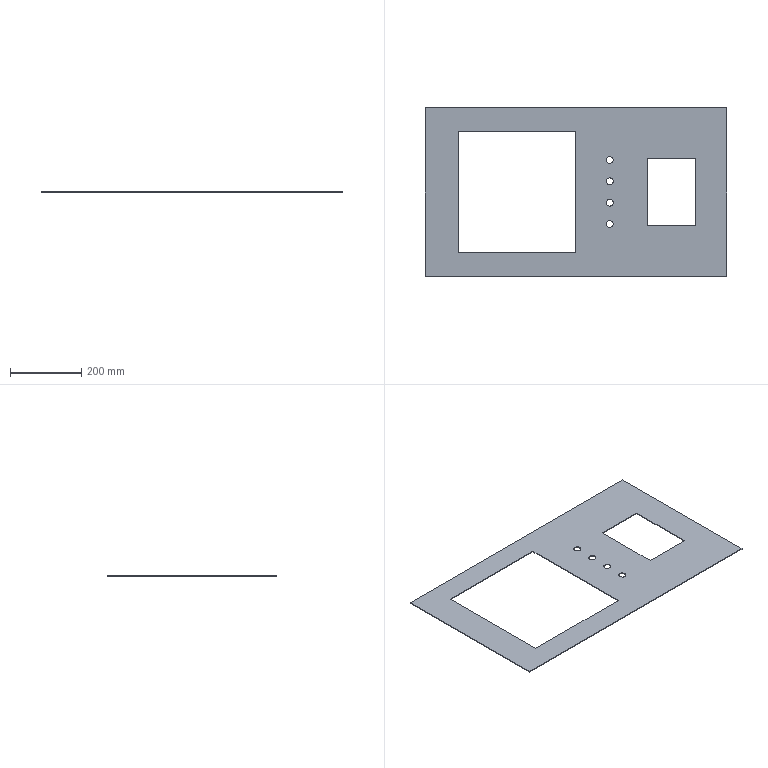Part | STEP file | Upper frame door panel | 1 solid | 22 faces | box 848 x 474.5 x 2 mm | volume 525505 mm3 | plane 14 | cylinder 8 | commonest cylinder face diameters 20 x8
STEP:
#1=CARTESIAN_POINT('',(105.,90.,0.));
#2=VERTEX_POINT('',#1);
#3=CARTESIAN_POINT('',(85.,90.,0.));
#4=VERTEX_POINT('',#3);
#5=CARTESIAN_POINT('',(95.,90.,0.));
#6=DIRECTION('',(0.,0.,-1.));
#7=DIRECTION('',(-1.,0.,0.));
#8=AXIS2_PLACEMENT_3D('',#5,#6,#7);
#9=CIRCLE('',#8,10.);
#10=EDGE_CURVE('',#2,#4,#9,.T.);
#11=ORIENTED_EDGE('',*,*,#10,.T.);
#12=CARTESIAN_POINT('',(85.,90.,2.));
#13=VERTEX_POINT('',#12);
#14=CARTESIAN_POINT('',(85.,90.,-0.001));
#15=DIRECTION('',(0.,0.,1.));
#16=VECTOR('',#15,1000.);
#17=LINE('',#14,#16);
#18=EDGE_CURVE('',#4,#13,#17,.T.);
#19=ORIENTED_EDGE('',*,*,#18,.T.);
#20=CARTESIAN_POINT('',(105.,90.,2.));
#21=VERTEX_POINT('',#20);
#22=CARTESIAN_POINT('',(95.,90.,2.));
#23=DIRECTION('',(0.,0.,-1.));
#24=DIRECTION('',(1.,0.,0.));
#25=AXIS2_PLACEMENT_3D('',#22,#23,#24);
#26=CIRCLE('',#25,10.);
#27=EDGE_CURVE('',#21,#13,#26,.T.);
#28=ORIENTED_EDGE('',*,*,#27,.F.);
#29=CARTESIAN_POINT('',(105.,90.,-0.001));
#30=DIRECTION('',(0.,0.,1.));
#31=VECTOR('',#30,1000.);
#32=LINE('',#29,#31);
#33=EDGE_CURVE('',#2,#21,#32,.T.);
#34=ORIENTED_EDGE('',*,*,#33,.F.);
#35=EDGE_LOOP('',(#11,#19,#28,#34));
#36=FACE_OUTER_BOUND('',#35,.T.);
#37=CARTESIAN_POINT('',(95.,90.,-0.001));
#38=DIRECTION('',(0.,0.,1.));
#39=DIRECTION('',(1.,0.,0.));
#40=AXIS2_PLACEMENT_3D('',#37,#38,#39);
#41=CYLINDRICAL_SURFACE('',#40,10.);
#42=ADVANCED_FACE('',(#36),#41,.F.);
#43=CARTESIAN_POINT('',(105.,30.,0.));
#44=VERTEX_POINT('',#43);
#45=CARTESIAN_POINT('',(85.,30.,0.));
#46=VERTEX_POINT('',#45);
#47=CARTESIAN_POINT('',(95.,30.,0.));
#48=DIRECTION('',(0.,0.,-1.));
#49=DIRECTION('',(-1.,0.,0.));
#50=AXIS2_PLACEMENT_3D('',#47,#48,#49);
#51=CIRCLE('',#50,10.);
#52=EDGE_CURVE('',#44,#46,#51,.T.);
#53=ORIENTED_EDGE('',*,*,#52,.T.);
#54=CARTESIAN_POINT('',(85.,30.,2.));
#55=VERTEX_POINT('',#54);
#56=CARTESIAN_POINT('',(85.,30.,-0.001));
#57=DIRECTION('',(0.,0.,1.));
#58=VECTOR('',#57,1000.);
#59=LINE('',#56,#58);
#60=EDGE_CURVE('',#46,#55,#59,.T.);
#61=ORIENTED_EDGE('',*,*,#60,.T.);
#62=CARTESIAN_POINT('',(105.,30.,2.));
#63=VERTEX_POINT('',#62);
#64=CARTESIAN_POINT('',(95.,30.,2.));
#65=DIRECTION('',(0.,0.,-1.));
#66=DIRECTION('',(1.,0.,0.));
#67=AXIS2_PLACEMENT_3D('',#64,#65,#66);
#68=CIRCLE('',#67,10.);
#69=EDGE_CURVE('',#63,#55,#68,.T.);
#70=ORIENTED_EDGE('',*,*,#69,.F.);
#71=CARTESIAN_POINT('',(105.,30.,-0.001));
#72=DIRECTION('',(0.,0.,1.));
#73=VECTOR('',#72,1000.);
#74=LINE('',#71,#73);
#75=EDGE_CURVE('',#44,#63,#74,.T.);
#76=ORIENTED_EDGE('',*,*,#75,.F.);
#77=EDGE_LOOP('',(#53,#61,#70,#76));
#78=FACE_OUTER_BOUND('',#77,.T.);
#79=CARTESIAN_POINT('',(95.,30.,-0.001));
#80=DIRECTION('',(0.,0.,1.));
#81=DIRECTION('',(1.,0.,0.));
#82=AXIS2_PLACEMENT_3D('',#79,#80,#81);
#83=CYLINDRICAL_SURFACE('',#82,10.);
#84=ADVANCED_FACE('',(#78),#83,.F.);
#85=CARTESIAN_POINT('',(85.,-30.,0.));
#86=VERTEX_POINT('',#85);
#87=CARTESIAN_POINT('',(105.,-30.,0.));
#88=VERTEX_POINT('',#87);
#89=CARTESIAN_POINT('',(95.,-30.,0.));
#90=DIRECTION('',(0.,0.,1.));
#91=DIRECTION('',(-1.,0.,0.));
#92=AXIS2_PLACEMENT_3D('',#89,#90,#91);
#93=CIRCLE('',#92,10.);
#94=EDGE_CURVE('',#86,#88,#93,.T.);
#95=ORIENTED_EDGE('',*,*,#94,.F.);
#96=CARTESIAN_POINT('',(85.,-30.,2.));
#97=VERTEX_POINT('',#96);
#98=CARTESIAN_POINT('',(85.,-30.,-0.001));
#99=DIRECTION('',(0.,0.,1.));
#100=VECTOR('',#99,1000.);
#101=LINE('',#98,#100);
#102=EDGE_CURVE('',#86,#97,#101,.T.);
#103=ORIENTED_EDGE('',*,*,#102,.T.);
#104=CARTESIAN_POINT('',(105.,-30.,2.));
#105=VERTEX_POINT('',#104);
#106=CARTESIAN_POINT('',(95.,-30.,2.));
#107=DIRECTION('',(0.,0.,1.));
#108=DIRECTION('',(1.,0.,0.));
#109=AXIS2_PLACEMENT_3D('',#106,#107,#108);
#110=CIRCLE('',#109,10.);
#111=EDGE_CURVE('',#97,#105,#110,.T.);
#112=ORIENTED_EDGE('',*,*,#111,.T.);
#113=CARTESIAN_POINT('',(105.,-30.,-0.001));
#114=DIRECTION('',(0.,0.,1.));
#115=VECTOR('',#114,1000.);
#116=LINE('',#113,#115);
#117=EDGE_CURVE('',#88,#105,#116,.T.);
#118=ORIENTED_EDGE('',*,*,#117,.F.);
#119=EDGE_LOOP('',(#95,#103,#112,#118));
#120=FACE_OUTER_BOUND('',#119,.T.);
#121=CARTESIAN_POINT('',(95.,-30.,-0.001));
#122=DIRECTION('',(0.,0.,1.));
#123=DIRECTION('',(1.,0.,0.));
#124=AXIS2_PLACEMENT_3D('',#121,#122,#123);
#125=CYLINDRICAL_SURFACE('',#124,10.);
#126=ADVANCED_FACE('',(#120),#125,.F.);
#127=CARTESIAN_POINT('',(85.,-90.,0.));
#128=VERTEX_POINT('',#127);
#129=CARTESIAN_POINT('',(105.,-90.,0.));
#130=VERTEX_POINT('',#129);
#131=CARTESIAN_POINT('',(95.,-90.,0.));
#132=DIRECTION('',(0.,0.,1.));
#133=DIRECTION('',(-1.,0.,0.));
#134=AXIS2_PLACEMENT_3D('',#131,#132,#133);
#135=CIRCLE('',#134,10.);
#136=EDGE_CURVE('',#128,#130,#135,.T.);
#137=ORIENTED_EDGE('',*,*,#136,.F.);
#138=CARTESIAN_POINT('',(85.,-90.,2.));
#139=VERTEX_POINT('',#138);
#140=CARTESIAN_POINT('',(85.,-90.,-0.001));
#141=DIRECTION('',(0.,0.,1.));
#142=VECTOR('',#141,1000.);
#143=LINE('',#140,#142);
#144=EDGE_CURVE('',#128,#139,#143,.T.);
#145=ORIENTED_EDGE('',*,*,#144,.T.);
#146=CARTESIAN_POINT('',(105.,-90.,2.));
#147=VERTEX_POINT('',#146);
#148=CARTESIAN_POINT('',(95.,-90.,2.));
#149=DIRECTION('',(0.,0.,1.));
#150=DIRECTION('',(1.,0.,0.));
#151=AXIS2_PLACEMENT_3D('',#148,#149,#150);
#152=CIRCLE('',#151,10.);
#153=EDGE_CURVE('',#139,#147,#152,.T.);
#154=ORIENTED_EDGE('',*,*,#153,.T.);
#155=CARTESIAN_POINT('',(105.,-90.,-0.001));
#156=DIRECTION('',(0.,0.,1.));
#157=VECTOR('',#156,1000.);
#158=LINE('',#155,#157);
#159=EDGE_CURVE('',#130,#147,#158,.T.);
#160=ORIENTED_EDGE('',*,*,#159,.F.);
#161=EDGE_LOOP('',(#137,#145,#154,#160));
#162=FACE_OUTER_BOUND('',#161,.T.);
#163=CARTESIAN_POINT('',(95.,-90.,-0.001));
#164=DIRECTION('',(0.,0.,1.));
#165=DIRECTION('',(1.,0.,0.));
#166=AXIS2_PLACEMENT_3D('',#163,#164,#165);
#167=CYLINDRICAL_SURFACE('',#166,10.);
#168=ADVANCED_FACE('',(#162),#167,.F.);
#169=CARTESIAN_POINT('',(-1.325,170.,2.));
#170=VERTEX_POINT('',#169);
#171=CARTESIAN_POINT('',(-331.325,170.,2.));
#172=VERTEX_POINT('',#171);
#173=CARTESIAN_POINT('',(-331.325,170.,2.));
#174=DIRECTION('',(-1.,0.,0.));
#175=VECTOR('',#174,1000.);
#176=LINE('',#173,#175);
#177=EDGE_CURVE('',#170,#172,#176,.T.);
#178=ORIENTED_EDGE('',*,*,#177,.F.);
#179=CARTESIAN_POINT('',(-1.325,-170.,2.));
#180=VERTEX_POINT('',#179);
#181=CARTESIAN_POINT('',(-1.325,170.,2.));
#182=DIRECTION('',(0.,1.,0.));
#183=VECTOR('',#182,1000.);
#184=LINE('',#181,#183);
#185=EDGE_CURVE('',#180,#170,#184,.T.);
#186=ORIENTED_EDGE('',*,*,#185,.F.);
#187=CARTESIAN_POINT('',(-331.325,-170.,2.));
#188=VERTEX_POINT('',#187);
#189=CARTESIAN_POINT('',(-331.325,-170.,2.));
#190=DIRECTION('',(1.,0.,0.));
#191=VECTOR('',#190,1000.);
#192=LINE('',#189,#191);
#193=EDGE_CURVE('',#188,#180,#192,.T.);
#194=ORIENTED_EDGE('',*,*,#193,.F.);
#195=CARTESIAN_POINT('',(-331.325,170.,2.));
#196=DIRECTION('',(0.,-1.,0.));
#197=VECTOR('',#196,1000.);
#198=LINE('',#195,#197);
#199=EDGE_CURVE('',#172,#188,#198,.T.);
#200=ORIENTED_EDGE('',*,*,#199,.F.);
#201=EDGE_LOOP('',(#178,#186,#194,#200));
#202=FACE_BOUND('',#201,.T.);
#203=ORIENTED_EDGE('',*,*,#27,.T.);
#204=CARTESIAN_POINT('',(95.,90.,2.));
#205=DIRECTION('',(0.,0.,-1.));
#206=DIRECTION('',(1.,0.,0.));
#207=AXIS2_PLACEMENT_3D('',#204,#205,#206);
#208=CIRCLE('',#207,10.);
#209=EDGE_CURVE('',#13,#21,#208,.T.);
#210=ORIENTED_EDGE('',*,*,#209,.T.);
#211=EDGE_LOOP('',(#203,#210));
#212=FACE_BOUND('',#211,.T.);
#213=ORIENTED_EDGE('',*,*,#69,.T.);
#214=CARTESIAN_POINT('',(95.,30.,2.));
#215=DIRECTION('',(0.,0.,-1.));
#216=DIRECTION('',(1.,0.,0.));
#217=AXIS2_PLACEMENT_3D('',#214,#215,#216);
#218=CIRCLE('',#217,10.);
#219=EDGE_CURVE('',#55,#63,#218,.T.);
#220=ORIENTED_EDGE('',*,*,#219,.T.);
#221=EDGE_LOOP('',(#213,#220));
#222=FACE_BOUND('',#221,.T.);
#223=CARTESIAN_POINT('',(424.,-237.25,2.));
#224=VERTEX_POINT('',#223);
#225=CARTESIAN_POINT('',(424.,237.25,2.));
#226=VERTEX_POINT('',#225);
#227=CARTESIAN_POINT('',(424.,-237.25,2.));
#228=DIRECTION('',(0.,1.,0.));
#229=VECTOR('',#228,1000.);
#230=LINE('',#227,#229);
#231=EDGE_CURVE('',#224,#226,#230,.T.);
#232=ORIENTED_EDGE('',*,*,#231,.T.);
#233=CARTESIAN_POINT('',(-424.,237.25,2.));
#234=VERTEX_POINT('',#233);
#235=CARTESIAN_POINT('',(-424.,237.25,2.));
#236=DIRECTION('',(-1.,0.,0.));
#237=VECTOR('',#236,1000.);
#238=LINE('',#235,#237);
#239=EDGE_CURVE('',#226,#234,#238,.T.);
#240=ORIENTED_EDGE('',*,*,#239,.T.);
#241=CARTESIAN_POINT('',(-424.,-237.25,2.));
#242=VERTEX_POINT('',#241);
#243=CARTESIAN_POINT('',(-424.,-237.25,2.));
#244=DIRECTION('',(0.,-1.,0.));
#245=VECTOR('',#244,1000.);
#246=LINE('',#243,#245);
#247=EDGE_CURVE('',#234,#242,#246,.T.);
#248=ORIENTED_EDGE('',*,*,#247,.T.);
#249=CARTESIAN_POINT('',(-424.,-237.25,2.));
#250=DIRECTION('',(1.,0.,0.));
#251=VECTOR('',#250,1000.);
#252=LINE('',#249,#251);
#253=EDGE_CURVE('',#242,#224,#252,.T.);
#254=ORIENTED_EDGE('',*,*,#253,.T.);
#255=EDGE_LOOP('',(#232,#240,#248,#254));
#256=FACE_OUTER_BOUND('',#255,.T.);
#257=CARTESIAN_POINT('',(95.,-90.,2.));
#258=DIRECTION('',(0.,0.,1.));
#259=DIRECTION('',(1.,0.,0.));
#260=AXIS2_PLACEMENT_3D('',#257,#258,#259);
#261=CIRCLE('',#260,10.);
#262=EDGE_CURVE('',#147,#139,#261,.T.);
#263=ORIENTED_EDGE('',*,*,#262,.F.);
#264=ORIENTED_EDGE('',*,*,#153,.F.);
#265=EDGE_LOOP('',(#263,#264));
#266=FACE_BOUND('',#265,.T.);
#267=CARTESIAN_POINT('',(95.,-30.,2.));
#268=DIRECTION('',(0.,0.,1.));
#269=DIRECTION('',(1.,0.,0.));
#270=AXIS2_PLACEMENT_3D('',#267,#268,#269);
#271=CIRCLE('',#270,10.);
#272=EDGE_CURVE('',#105,#97,#271,.T.);
#273=ORIENTED_EDGE('',*,*,#272,.F.);
#274=ORIENTED_EDGE('',*,*,#111,.F.);
#275=EDGE_LOOP('',(#273,#274));
#276=FACE_BOUND('',#275,.T.);
#277=CARTESIAN_POINT('',(337.,95.5,2.));
#278=VERTEX_POINT('',#277);
#279=CARTESIAN_POINT('',(337.,-95.5,2.));
#280=VERTEX_POINT('',#279);
#281=CARTESIAN_POINT('',(337.,0.,2.));
#282=DIRECTION('',(0.,-1.,0.));
#283=VECTOR('',#282,1000.);
#284=LINE('',#281,#283);
#285=EDGE_CURVE('',#278,#280,#284,.T.);
#286=ORIENTED_EDGE('',*,*,#285,.T.);
#287=CARTESIAN_POINT('',(200.,-95.5,2.));
#288=VERTEX_POINT('',#287);
#289=CARTESIAN_POINT('',(0.,-95.5,2.));
#290=DIRECTION('',(1.,0.,0.));
#291=VECTOR('',#290,1000.);
#292=LINE('',#289,#291);
#293=EDGE_CURVE('',#288,#280,#292,.T.);
#294=ORIENTED_EDGE('',*,*,#293,.F.);
#295=CARTESIAN_POINT('',(200.,95.5,2.));
#296=VERTEX_POINT('',#295);
#297=CARTESIAN_POINT('',(200.,0.,2.));
#298=DIRECTION('',(0.,-1.,0.));
#299=VECTOR('',#298,1000.);
#300=LINE('',#297,#299);
#301=EDGE_CURVE('',#296,#288,#300,.T.);
#302=ORIENTED_EDGE('',*,*,#301,.F.);
#303=CARTESIAN_POINT('',(0.,95.5,2.));
#304=DIRECTION('',(1.,0.,0.));
#305=VECTOR('',#304,1000.);
#306=LINE('',#303,#305);
#307=EDGE_CURVE('',#296,#278,#306,.T.);
#308=ORIENTED_EDGE('',*,*,#307,.T.);
#309=EDGE_LOOP('',(#286,#294,#302,#308));
#310=FACE_BOUND('',#309,.T.);
#311=CARTESIAN_POINT('',(0.,0.,2.));
#312=DIRECTION('',(0.,0.,-1.));
#313=DIRECTION('',(-1.,0.,0.));
#314=AXIS2_PLACEMENT_3D('',#311,#312,#313);
#315=PLANE('',#314);
#316=ADVANCED_FACE('',(#202,#212,#222,#256,#266,#276,#310),#315,.F.);
#317=CARTESIAN_POINT('',(-1.325,-170.,0.));
#318=VERTEX_POINT('',#317);
#319=CARTESIAN_POINT('',(-1.325,170.,0.));
#320=VERTEX_POINT('',#319);
#321=CARTESIAN_POINT('',(-1.325,170.,0.));
#322=DIRECTION('',(0.,1.,0.));
#323=VECTOR('',#322,1000.);
#324=LINE('',#321,#323);
#325=EDGE_CURVE('',#318,#320,#324,.T.);
#326=ORIENTED_EDGE('',*,*,#325,.T.);
#327=CARTESIAN_POINT('',(-331.325,170.,0.));
#328=VERTEX_POINT('',#327);
#329=CARTESIAN_POINT('',(-331.325,170.,0.));
#330=DIRECTION('',(-1.,0.,0.));
#331=VECTOR('',#330,1000.);
#332=LINE('',#329,#331);
#333=EDGE_CURVE('',#320,#328,#332,.T.);
#334=ORIENTED_EDGE('',*,*,#333,.T.);
#335=CARTESIAN_POINT('',(-331.325,-170.,0.));
#336=VERTEX_POINT('',#335);
#337=CARTESIAN_POINT('',(-331.325,170.,0.));
#338=DIRECTION('',(0.,-1.,0.));
#339=VECTOR('',#338,1000.);
#340=LINE('',#337,#339);
#341=EDGE_CURVE('',#328,#336,#340,.T.);
#342=ORIENTED_EDGE('',*,*,#341,.T.);
#343=CARTESIAN_POINT('',(-331.325,-170.,0.));
#344=DIRECTION('',(1.,0.,0.));
#345=VECTOR('',#344,1000.);
#346=LINE('',#343,#345);
#347=EDGE_CURVE('',#336,#318,#346,.T.);
#348=ORIENTED_EDGE('',*,*,#347,.T.);
#349=EDGE_LOOP('',(#326,#334,#342,#348));
#350=FACE_BOUND('',#349,.T.);
#351=ORIENTED_EDGE('',*,*,#52,.F.);
#352=CARTESIAN_POINT('',(95.,30.,0.));
#353=DIRECTION('',(0.,0.,-1.));
#354=DIRECTION('',(-1.,0.,0.));
#355=AXIS2_PLACEMENT_3D('',#352,#353,#354);
#356=CIRCLE('',#355,10.);
#357=EDGE_CURVE('',#46,#44,#356,.T.);
#358=ORIENTED_EDGE('',*,*,#357,.F.);
#359=EDGE_LOOP('',(#351,#358));
#360=FACE_BOUND('',#359,.T.);
#361=CARTESIAN_POINT('',(95.,-30.,0.));
#362=DIRECTION('',(0.,0.,1.));
#363=DIRECTION('',(-1.,0.,0.));
#364=AXIS2_PLACEMENT_3D('',#361,#362,#363);
#365=CIRCLE('',#364,10.);
#366=EDGE_CURVE('',#88,#86,#365,.T.);
#367=ORIENTED_EDGE('',*,*,#366,.T.);
#368=ORIENTED_EDGE('',*,*,#94,.T.);
#369=EDGE_LOOP('',(#367,#368));
#370=FACE_BOUND('',#369,.T.);
#371=CARTESIAN_POINT('',(95.,-90.,0.));
#372=DIRECTION('',(0.,0.,1.));
#373=DIRECTION('',(-1.,0.,0.));
#374=AXIS2_PLACEMENT_3D('',#371,#372,#373);
#375=CIRCLE('',#374,10.);
#376=EDGE_CURVE('',#130,#128,#375,.T.);
#377=ORIENTED_EDGE('',*,*,#376,.T.);
#378=ORIENTED_EDGE('',*,*,#136,.T.);
#379=EDGE_LOOP('',(#377,#378));
#380=FACE_BOUND('',#379,.T.);
#381=CARTESIAN_POINT('',(424.,-237.25,0.));
#382=VERTEX_POINT('',#381);
#383=CARTESIAN_POINT('',(424.,237.25,0.));
#384=VERTEX_POINT('',#383);
#385=CARTESIAN_POINT('',(424.,-237.25,0.));
#386=DIRECTION('',(0.,1.,0.));
#387=VECTOR('',#386,1000.);
#388=LINE('',#385,#387);
#389=EDGE_CURVE('',#382,#384,#388,.T.);
#390=ORIENTED_EDGE('',*,*,#389,.F.);
#391=CARTESIAN_POINT('',(-424.,-237.25,0.));
#392=VERTEX_POINT('',#391);
#393=CARTESIAN_POINT('',(-424.,-237.25,0.));
#394=DIRECTION('',(1.,0.,0.));
#395=VECTOR('',#394,1000.);
#396=LINE('',#393,#395);
#397=EDGE_CURVE('',#392,#382,#396,.T.);
#398=ORIENTED_EDGE('',*,*,#397,.F.);
#399=CARTESIAN_POINT('',(-424.,237.25,0.));
#400=VERTEX_POINT('',#399);
#401=CARTESIAN_POINT('',(-424.,-237.25,0.));
#402=DIRECTION('',(0.,-1.,0.));
#403=VECTOR('',#402,1000.);
#404=LINE('',#401,#403);
#405=EDGE_CURVE('',#400,#392,#404,.T.);
#406=ORIENTED_EDGE('',*,*,#405,.F.);
#407=CARTESIAN_POINT('',(-424.,237.25,0.));
#408=DIRECTION('',(-1.,0.,0.));
#409=VECTOR('',#408,1000.);
#410=LINE('',#407,#409);
#411=EDGE_CURVE('',#384,#400,#410,.T.);
#412=ORIENTED_EDGE('',*,*,#411,.F.);
#413=EDGE_LOOP('',(#390,#398,#406,#412));
#414=FACE_OUTER_BOUND('',#413,.T.);
#415=ORIENTED_EDGE('',*,*,#10,.F.);
#416=CARTESIAN_POINT('',(95.,90.,0.));
#417=DIRECTION('',(0.,0.,-1.));
#418=DIRECTION('',(-1.,0.,0.));
#419=AXIS2_PLACEMENT_3D('',#416,#417,#418);
#420=CIRCLE('',#419,10.);
#421=EDGE_CURVE('',#4,#2,#420,.T.);
#422=ORIENTED_EDGE('',*,*,#421,.F.);
#423=EDGE_LOOP('',(#415,#422));
#424=FACE_BOUND('',#423,.T.);
#425=CARTESIAN_POINT('',(200.,-95.5,0.));
#426=VERTEX_POINT('',#425);
#427=CARTESIAN_POINT('',(337.,-95.5,0.));
#428=VERTEX_POINT('',#427);
#429=CARTESIAN_POINT('',(0.,-95.5,0.));
#430=DIRECTION('',(1.,0.,0.));
#431=VECTOR('',#430,1000.);
#432=LINE('',#429,#431);
#433=EDGE_CURVE('',#426,#428,#432,.T.);
#434=ORIENTED_EDGE('',*,*,#433,.T.);
#435=CARTESIAN_POINT('',(337.,95.5,0.));
#436=VERTEX_POINT('',#435);
#437=CARTESIAN_POINT('',(337.,0.,0.));
#438=DIRECTION('',(0.,-1.,0.));
#439=VECTOR('',#438,1000.);
#440=LINE('',#437,#439);
#441=EDGE_CURVE('',#436,#428,#440,.T.);
#442=ORIENTED_EDGE('',*,*,#441,.F.);
#443=CARTESIAN_POINT('',(200.,95.5,0.));
#444=VERTEX_POINT('',#443);
#445=CARTESIAN_POINT('',(0.,95.5,0.));
#446=DIRECTION('',(1.,0.,0.));
#447=VECTOR('',#446,1000.);
#448=LINE('',#445,#447);
#449=EDGE_CURVE('',#444,#436,#448,.T.);
#450=ORIENTED_EDGE('',*,*,#449,.F.);
#451=CARTESIAN_POINT('',(200.,0.,0.));
#452=DIRECTION('',(0.,-1.,0.));
#453=VECTOR('',#452,1000.);
#454=LINE('',#451,#453);
#455=EDGE_CURVE('',#444,#426,#454,.T.);
#456=ORIENTED_EDGE('',*,*,#455,.T.);
#457=EDGE_LOOP('',(#434,#442,#450,#456));
#458=FACE_BOUND('',#457,.T.);
#459=CARTESIAN_POINT('',(0.,0.,0.));
#460=DIRECTION('',(0.,0.,-1.));
#461=DIRECTION('',(-1.,0.,0.));
#462=AXIS2_PLACEMENT_3D('',#459,#460,#461);
#463=PLANE('',#462);
#464=ADVANCED_FACE('',(#350,#360,#370,#380,#414,#424,#458),#463,.T.);
#465=ORIENTED_EDGE('',*,*,#389,.T.);
#466=CARTESIAN_POINT('',(424.,237.25,2.));
#467=DIRECTION('',(0.,0.,-1.));
#468=VECTOR('',#467,1000.);
#469=LINE('',#466,#468);
#470=EDGE_CURVE('',#226,#384,#469,.T.);
#471=ORIENTED_EDGE('',*,*,#470,.F.);
#472=ORIENTED_EDGE('',*,*,#231,.F.);
#473=CARTESIAN_POINT('',(424.,-237.25,2.));
#474=DIRECTION('',(0.,0.,-1.));
#475=VECTOR('',#474,1000.);
#476=LINE('',#473,#475);
#477=EDGE_CURVE('',#224,#382,#476,.T.);
#478=ORIENTED_EDGE('',*,*,#477,.T.);
#479=EDGE_LOOP('',(#465,#471,#472,#478));
#480=FACE_OUTER_BOUND('',#479,.T.);
#481=CARTESIAN_POINT('',(424.,-237.25,2.));
#482=DIRECTION('',(-1.,0.,0.));
#483=DIRECTION('',(0.,0.,1.));
#484=AXIS2_PLACEMENT_3D('',#481,#482,#483);
#485=PLANE('',#484);
#486=ADVANCED_FACE('',(#480),#485,.F.);
#487=ORIENTED_EDGE('',*,*,#411,.T.);
#488=CARTESIAN_POINT('',(-424.,237.25,2.));
#489=DIRECTION('',(0.,0.,-1.));
#490=VECTOR('',#489,1000.);
#491=LINE('',#488,#490);
#492=EDGE_CURVE('',#234,#400,#491,.T.);
#493=ORIENTED_EDGE('',*,*,#492,.F.);
#494=ORIENTED_EDGE('',*,*,#239,.F.);
#495=ORIENTED_EDGE('',*,*,#470,.T.);
#496=EDGE_LOOP('',(#487,#493,#494,#495));
#497=FACE_OUTER_BOUND('',#496,.T.);
#498=CARTESIAN_POINT('',(-424.,237.25,2.));
#499=DIRECTION('',(0.,-1.,0.));
#500=DIRECTION('',(0.,0.,-1.));
#501=AXIS2_PLACEMENT_3D('',#498,#499,#500);
#502=PLANE('',#501);
#503=ADVANCED_FACE('',(#497),#502,.F.);
#504=ORIENTED_EDGE('',*,*,#405,.T.);
#505=CARTESIAN_POINT('',(-424.,-237.25,2.));
#506=DIRECTION('',(0.,0.,-1.));
#507=VECTOR('',#506,1000.);
#508=LINE('',#505,#507);
#509=EDGE_CURVE('',#242,#392,#508,.T.);
#510=ORIENTED_EDGE('',*,*,#509,.F.);
#511=ORIENTED_EDGE('',*,*,#247,.F.);
#512=ORIENTED_EDGE('',*,*,#492,.T.);
#513=EDGE_LOOP('',(#504,#510,#511,#512));
#514=FACE_OUTER_BOUND('',#513,.T.);
#515=CARTESIAN_POINT('',(-424.,-237.25,2.));
#516=DIRECTION('',(1.,0.,0.));
#517=DIRECTION('',(0.,1.,0.));
#518=AXIS2_PLACEMENT_3D('',#515,#516,#517);
#519=PLANE('',#518);
#520=ADVANCED_FACE('',(#514),#519,.F.);
#521=ORIENTED_EDGE('',*,*,#397,.T.);
#522=ORIENTED_EDGE('',*,*,#477,.F.);
#523=ORIENTED_EDGE('',*,*,#253,.F.);
#524=ORIENTED_EDGE('',*,*,#509,.T.);
#525=EDGE_LOOP('',(#521,#522,#523,#524));
#526=FACE_OUTER_BOUND('',#525,.T.);
#527=CARTESIAN_POINT('',(-424.,-237.25,2.));
#528=DIRECTION('',(0.,1.,0.));
#529=DIRECTION('',(0.,0.,1.));
#530=AXIS2_PLACEMENT_3D('',#527,#528,#529);
#531=PLANE('',#530);
#532=ADVANCED_FACE('',(#526),#531,.F.);
#533=ORIENTED_EDGE('',*,*,#144,.F.);
#534=ORIENTED_EDGE('',*,*,#376,.F.);
#535=ORIENTED_EDGE('',*,*,#159,.T.);
#536=ORIENTED_EDGE('',*,*,#262,.T.);
#537=EDGE_LOOP('',(#533,#534,#535,#536));
#538=FACE_OUTER_BOUND('',#537,.T.);
#539=CARTESIAN_POINT('',(95.,-90.,-0.001));
#540=DIRECTION('',(0.,0.,1.));
#541=DIRECTION('',(1.,0.,0.));
#542=AXIS2_PLACEMENT_3D('',#539,#540,#541);
#543=CYLINDRICAL_SURFACE('',#542,10.);
#544=ADVANCED_FACE('',(#538),#543,.F.);
#545=ORIENTED_EDGE('',*,*,#102,.F.);
#546=ORIENTED_EDGE('',*,*,#366,.F.);
#547=ORIENTED_EDGE('',*,*,#117,.T.);
#548=ORIENTED_EDGE('',*,*,#272,.T.);
#549=EDGE_LOOP('',(#545,#546,#547,#548));
#550=FACE_OUTER_BOUND('',#549,.T.);
#551=CARTESIAN_POINT('',(95.,-30.,-0.001));
#552=DIRECTION('',(0.,0.,1.));
#553=DIRECTION('',(1.,0.,0.));
#554=AXIS2_PLACEMENT_3D('',#551,#552,#553);
#555=CYLINDRICAL_SURFACE('',#554,10.);
#556=ADVANCED_FACE('',(#550),#555,.F.);
#557=ORIENTED_EDGE('',*,*,#60,.F.);
#558=ORIENTED_EDGE('',*,*,#357,.T.);
#559=ORIENTED_EDGE('',*,*,#75,.T.);
#560=ORIENTED_EDGE('',*,*,#219,.F.);
#561=EDGE_LOOP('',(#557,#558,#559,#560));
#562=FACE_OUTER_BOUND('',#561,.T.);
#563=CARTESIAN_POINT('',(95.,30.,-0.001));
#564=DIRECTION('',(0.,0.,1.));
#565=DIRECTION('',(1.,0.,0.));
#566=AXIS2_PLACEMENT_3D('',#563,#564,#565);
#567=CYLINDRICAL_SURFACE('',#566,10.);
#568=ADVANCED_FACE('',(#562),#567,.F.);
#569=ORIENTED_EDGE('',*,*,#18,.F.);
#570=ORIENTED_EDGE('',*,*,#421,.T.);
#571=ORIENTED_EDGE('',*,*,#33,.T.);
#572=ORIENTED_EDGE('',*,*,#209,.F.);
#573=EDGE_LOOP('',(#569,#570,#571,#572));
#574=FACE_OUTER_BOUND('',#573,.T.);
#575=CARTESIAN_POINT('',(95.,90.,-0.001));
#576=DIRECTION('',(0.,0.,1.));
#577=DIRECTION('',(1.,0.,0.));
#578=AXIS2_PLACEMENT_3D('',#575,#576,#577);
#579=CYLINDRICAL_SURFACE('',#578,10.);
#580=ADVANCED_FACE('',(#574),#579,.F.);
#581=ORIENTED_EDGE('',*,*,#441,.T.);
#582=CARTESIAN_POINT('',(337.,-95.5,-0.001));
#583=DIRECTION('',(0.,0.,1.));
#584=VECTOR('',#583,1000.);
#585=LINE('',#582,#584);
#586=EDGE_CURVE('',#428,#280,#585,.T.);
#587=ORIENTED_EDGE('',*,*,#586,.T.);
#588=ORIENTED_EDGE('',*,*,#285,.F.);
#589=CARTESIAN_POINT('',(337.,95.5,-0.001));
#590=DIRECTION('',(0.,0.,1.));
#591=VECTOR('',#590,1000.);
#592=LINE('',#589,#591);
#593=EDGE_CURVE('',#436,#278,#592,.T.);
#594=ORIENTED_EDGE('',*,*,#593,.F.);
#595=EDGE_LOOP('',(#581,#587,#588,#594));
#596=FACE_OUTER_BOUND('',#595,.T.);
#597=CARTESIAN_POINT('',(337.,0.,-0.001));
#598=DIRECTION('',(-1.,0.,0.));
#599=DIRECTION('',(0.,0.,1.));
#600=AXIS2_PLACEMENT_3D('',#597,#598,#599);
#601=PLANE('',#600);
#602=ADVANCED_FACE('',(#596),#601,.T.);
#603=CARTESIAN_POINT('',(200.,-95.5,-0.001));
#604=DIRECTION('',(0.,0.,1.));
#605=VECTOR('',#604,1000.);
#606=LINE('',#603,#605);
#607=EDGE_CURVE('',#426,#288,#606,.T.);
#608=ORIENTED_EDGE('',*,*,#607,.T.);
#609=ORIENTED_EDGE('',*,*,#293,.T.);
#610=ORIENTED_EDGE('',*,*,#586,.F.);
#611=ORIENTED_EDGE('',*,*,#433,.F.);
#612=EDGE_LOOP('',(#608,#609,#610,#611));
#613=FACE_OUTER_BOUND('',#612,.T.);
#614=CARTESIAN_POINT('',(0.,-95.5,-0.001));
#615=DIRECTION('',(0.,-1.,0.));
#616=DIRECTION('',(0.,0.,-1.));
#617=AXIS2_PLACEMENT_3D('',#614,#615,#616);
#618=PLANE('',#617);
#619=ADVANCED_FACE('',(#613),#618,.F.);
#620=CARTESIAN_POINT('',(200.,95.5,-0.001));
#621=DIRECTION('',(0.,0.,1.));
#622=VECTOR('',#621,1000.);
#623=LINE('',#620,#622);
#624=EDGE_CURVE('',#444,#296,#623,.T.);
#625=ORIENTED_EDGE('',*,*,#624,.T.);
#626=ORIENTED_EDGE('',*,*,#301,.T.);
#627=ORIENTED_EDGE('',*,*,#607,.F.);
#628=ORIENTED_EDGE('',*,*,#455,.F.);
#629=EDGE_LOOP('',(#625,#626,#627,#628));
#630=FACE_OUTER_BOUND('',#629,.T.);
#631=CARTESIAN_POINT('',(200.,0.,-0.001));
#632=DIRECTION('',(-1.,0.,0.));
#633=DIRECTION('',(0.,0.,1.));
#634=AXIS2_PLACEMENT_3D('',#631,#632,#633);
#635=PLANE('',#634);
#636=ADVANCED_FACE('',(#630),#635,.F.);
#637=ORIENTED_EDGE('',*,*,#449,.T.);
#638=ORIENTED_EDGE('',*,*,#593,.T.);
#639=ORIENTED_EDGE('',*,*,#307,.F.);
#640=ORIENTED_EDGE('',*,*,#624,.F.);
#641=EDGE_LOOP('',(#637,#638,#639,#640));
#642=FACE_OUTER_BOUND('',#641,.T.);
#643=CARTESIAN_POINT('',(0.,95.5,-0.001));
#644=DIRECTION('',(0.,-1.,0.));
#645=DIRECTION('',(0.,0.,-1.));
#646=AXIS2_PLACEMENT_3D('',#643,#644,#645);
#647=PLANE('',#646);
#648=ADVANCED_FACE('',(#642),#647,.T.);
#649=CARTESIAN_POINT('',(-1.325,-170.,-0.001));
#650=DIRECTION('',(0.,0.,1.));
#651=VECTOR('',#650,1000.);
#652=LINE('',#649,#651);
#653=EDGE_CURVE('',#318,#180,#652,.T.);
#654=ORIENTED_EDGE('',*,*,#653,.T.);
#655=ORIENTED_EDGE('',*,*,#185,.T.);
#656=CARTESIAN_POINT('',(-1.325,170.,-0.001));
#657=DIRECTION('',(0.,0.,1.));
#658=VECTOR('',#657,1000.);
#659=LINE('',#656,#658);
#660=EDGE_CURVE('',#320,#170,#659,.T.);
#661=ORIENTED_EDGE('',*,*,#660,.F.);
#662=ORIENTED_EDGE('',*,*,#325,.F.);
#663=EDGE_LOOP('',(#654,#655,#661,#662));
#664=FACE_OUTER_BOUND('',#663,.T.);
#665=CARTESIAN_POINT('',(-1.325,170.,-0.001));
#666=DIRECTION('',(1.,0.,0.));
#667=DIRECTION('',(0.,0.,-1.));
#668=AXIS2_PLACEMENT_3D('',#665,#666,#667);
#669=PLANE('',#668);
#670=ADVANCED_FACE('',(#664),#669,.F.);
#671=CARTESIAN_POINT('',(-331.325,-170.,-0.001));
#672=DIRECTION('',(0.,0.,1.));
#673=VECTOR('',#672,1000.);
#674=LINE('',#671,#673);
#675=EDGE_CURVE('',#336,#188,#674,.T.);
#676=ORIENTED_EDGE('',*,*,#675,.T.);
#677=ORIENTED_EDGE('',*,*,#193,.T.);
#678=ORIENTED_EDGE('',*,*,#653,.F.);
#679=ORIENTED_EDGE('',*,*,#347,.F.);
#680=EDGE_LOOP('',(#676,#677,#678,#679));
#681=FACE_OUTER_BOUND('',#680,.T.);
#682=CARTESIAN_POINT('',(-331.325,-170.,-0.001));
#683=DIRECTION('',(0.,-1.,0.));
#684=DIRECTION('',(1.,0.,0.));
#685=AXIS2_PLACEMENT_3D('',#682,#683,#684);
#686=PLANE('',#685);
#687=ADVANCED_FACE('',(#681),#686,.F.);
#688=CARTESIAN_POINT('',(-331.325,170.,-0.001));
#689=DIRECTION('',(0.,0.,1.));
#690=VECTOR('',#689,1000.);
#691=LINE('',#688,#690);
#692=EDGE_CURVE('',#328,#172,#691,.T.);
#693=ORIENTED_EDGE('',*,*,#692,.T.);
#694=ORIENTED_EDGE('',*,*,#199,.T.);
#695=ORIENTED_EDGE('',*,*,#675,.F.);
#696=ORIENTED_EDGE('',*,*,#341,.F.);
#697=EDGE_LOOP('',(#693,#694,#695,#696));
#698=FACE_OUTER_BOUND('',#697,.T.);
#699=CARTESIAN_POINT('',(-331.325,170.,-0.001));
#700=DIRECTION('',(-1.,0.,0.));
#701=DIRECTION('',(0.,0.,1.));
#702=AXIS2_PLACEMENT_3D('',#699,#700,#701);
#703=PLANE('',#702);
#704=ADVANCED_FACE('',(#698),#703,.F.);
#705=ORIENTED_EDGE('',*,*,#660,.T.);
#706=ORIENTED_EDGE('',*,*,#177,.T.);
#707=ORIENTED_EDGE('',*,*,#692,.F.);
#708=ORIENTED_EDGE('',*,*,#333,.F.);
#709=EDGE_LOOP('',(#705,#706,#707,#708));
#710=FACE_OUTER_BOUND('',#709,.T.);
#711=CARTESIAN_POINT('',(-331.325,170.,-0.001));
#712=DIRECTION('',(0.,1.,0.));
#713=DIRECTION('',(0.,0.,1.));
#714=AXIS2_PLACEMENT_3D('',#711,#712,#713);
#715=PLANE('',#714);
#716=ADVANCED_FACE('',(#710),#715,.F.);
#717=CLOSED_SHELL('',(#42,#84,#126,#168,#316,#464,#486,#503,#520,#532,#544,#556,#568,#580,#602,#619,#636,#648,#670,#687,#704,#716));
#718=MANIFOLD_SOLID_BREP('',#717);
#719=CARTESIAN_POINT('',(0.,0.,0.));
#720=DIRECTION('',(0.,0.,1.));
#721=DIRECTION('',(1.,0.,0.));
#722=AXIS2_PLACEMENT_3D('',#719,#720,#721);
#723=(LENGTH_UNIT()NAMED_UNIT(*)SI_UNIT(.MILLI.,.METRE.));
#724=UNCERTAINTY_MEASURE_WITH_UNIT(LENGTH_MEASURE(0.00001),#723,'','');
#725=(NAMED_UNIT(*)PLANE_ANGLE_UNIT()SI_UNIT($,.RADIAN.));
#726=(NAMED_UNIT(*)SI_UNIT($,.STERADIAN.)SOLID_ANGLE_UNIT());
#727=(GEOMETRIC_REPRESENTATION_CONTEXT(3)GLOBAL_UNCERTAINTY_ASSIGNED_CONTEXT((#724))GLOBAL_UNIT_ASSIGNED_CONTEXT((#723,#725,#726))REPRESENTATION_CONTEXT('',''));
#728=ADVANCED_BREP_SHAPE_REPRESENTATION('',(#718,#722),#727);